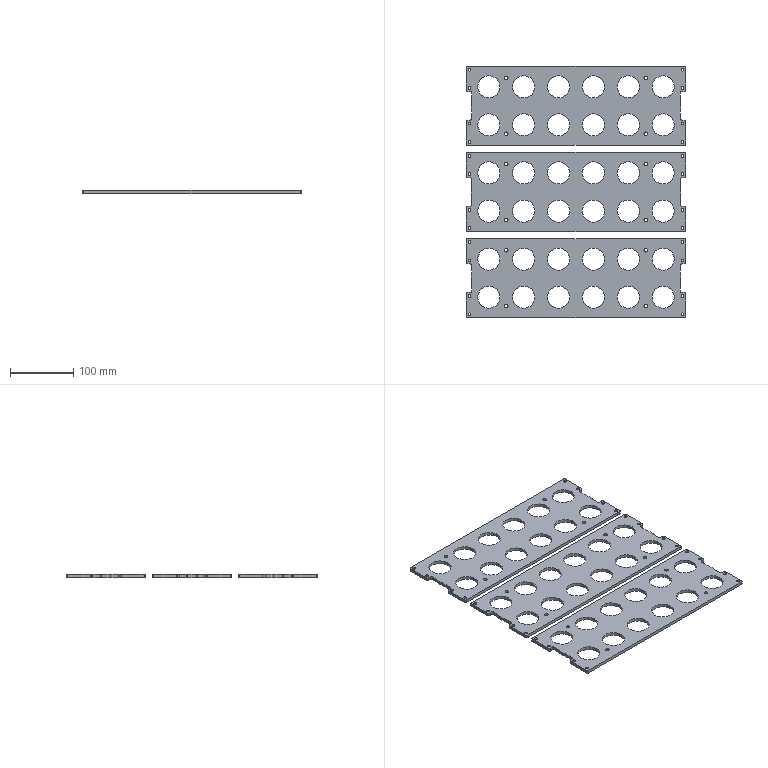Part | 3 solids | 987 faces | box 346 x 397 x 5 mm | volume 459115 mm3 | plane 501 | cylinder 342 | spline 120 | cone 24 | commonest cylinder face diameters 2.699 x60 4 x36 35 x36 1 x24 3.3 x24 4.5 x24